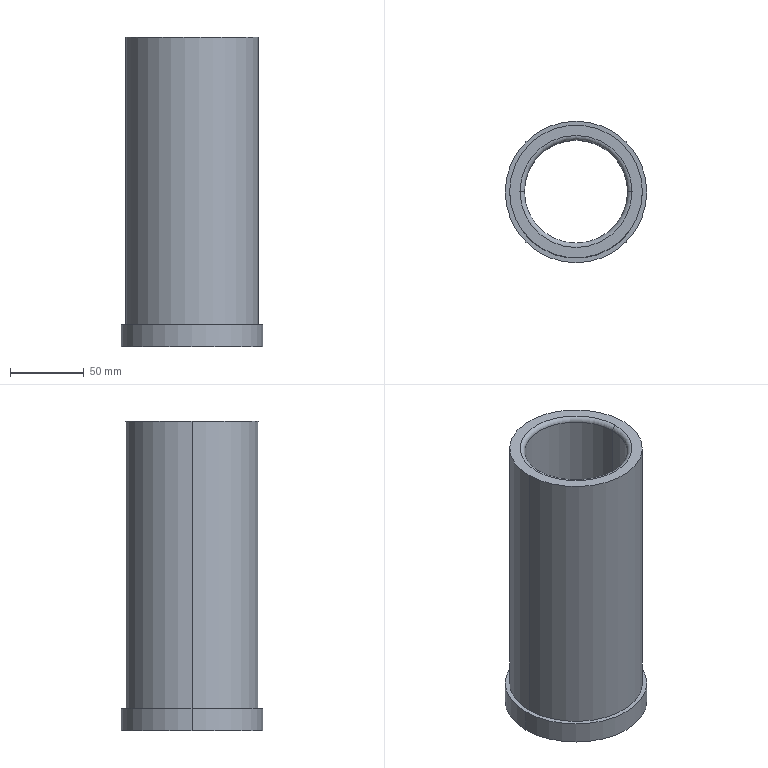Part | SolidWorks | features BaseBody 1 | 1 solid | 13 faces | box 96 x 96 x 210 mm | volume 540069 mm3 | cylinder 6 | torus 4 | plane 3 | commonest cylinder face diameters 70 x2 90 x2 96 x2
STEP:
#1=CARTESIAN_POINT('',(-383.,-275.,-0.5));
#2=VERTEX_POINT('',#1);
#3=CARTESIAN_POINT('',(-307.,-275.,-0.5));
#4=VERTEX_POINT('',#3);
#5=CARTESIAN_POINT('',(-345.,-275.,-0.5));
#6=DIRECTION('',(0.,0.,-1.));
#7=DIRECTION('',(1.,0.,0.));
#8=AXIS2_PLACEMENT_3D('',#5,#6,#7);
#9=CIRCLE('',#8,38.);
#10=EDGE_CURVE('',#2,#4,#9,.T.);
#11=ORIENTED_EDGE('',*,*,#10,.F.);
#12=CARTESIAN_POINT('',(-380.,-275.,-3.5));
#13=VERTEX_POINT('',#12);
#14=CARTESIAN_POINT('',(-383.,-275.,-3.5));
#15=DIRECTION('',(0.,1.,0.));
#16=DIRECTION('',(-1.,0.,0.));
#17=AXIS2_PLACEMENT_3D('',#14,#15,#16);
#18=CIRCLE('',#17,3.);
#19=EDGE_CURVE('',#2,#13,#18,.T.);
#20=ORIENTED_EDGE('',*,*,#19,.T.);
#21=CARTESIAN_POINT('',(-310.,-275.,-3.5));
#22=VERTEX_POINT('',#21);
#23=CARTESIAN_POINT('',(-345.,-275.,-3.5));
#24=DIRECTION('',(0.,0.,1.));
#25=DIRECTION('',(1.,0.,0.));
#26=AXIS2_PLACEMENT_3D('',#23,#24,#25);
#27=CIRCLE('',#26,35.);
#28=EDGE_CURVE('',#22,#13,#27,.T.);
#29=ORIENTED_EDGE('',*,*,#28,.F.);
#30=CARTESIAN_POINT('',(-307.,-275.,-3.5));
#31=DIRECTION('',(0.,-1.,0.));
#32=DIRECTION('',(0.,0.,-1.));
#33=AXIS2_PLACEMENT_3D('',#30,#31,#32);
#34=CIRCLE('',#33,3.);
#35=EDGE_CURVE('',#4,#22,#34,.T.);
#36=ORIENTED_EDGE('',*,*,#35,.F.);
#37=EDGE_LOOP('',(#11,#20,#29,#36));
#38=FACE_OUTER_BOUND('',#37,.T.);
#39=CARTESIAN_POINT('',(-345.,-275.,-3.5));
#40=DIRECTION('',(0.,0.,1.));
#41=DIRECTION('',(1.,0.,0.));
#42=AXIS2_PLACEMENT_3D('',#39,#40,#41);
#43=TOROIDAL_SURFACE('',#42,38.,3.);
#44=ADVANCED_FACE('',(#38),#43,.T.);
#45=CARTESIAN_POINT('',(-380.,-275.,-207.5));
#46=VERTEX_POINT('',#45);
#47=CARTESIAN_POINT('',(-310.,-275.,-207.5));
#48=VERTEX_POINT('',#47);
#49=CARTESIAN_POINT('',(-345.,-275.,-207.5));
#50=DIRECTION('',(0.,0.,-1.));
#51=DIRECTION('',(1.,0.,0.));
#52=AXIS2_PLACEMENT_3D('',#49,#50,#51);
#53=CIRCLE('',#52,35.);
#54=EDGE_CURVE('',#46,#48,#53,.T.);
#55=ORIENTED_EDGE('',*,*,#54,.F.);
#56=CARTESIAN_POINT('',(-383.,-275.,-210.5));
#57=VERTEX_POINT('',#56);
#58=CARTESIAN_POINT('',(-383.,-275.,-207.5));
#59=DIRECTION('',(0.,1.,0.));
#60=DIRECTION('',(-1.,0.,0.));
#61=AXIS2_PLACEMENT_3D('',#58,#59,#60);
#62=CIRCLE('',#61,3.);
#63=EDGE_CURVE('',#46,#57,#62,.T.);
#64=ORIENTED_EDGE('',*,*,#63,.T.);
#65=CARTESIAN_POINT('',(-307.,-275.,-210.5));
#66=VERTEX_POINT('',#65);
#67=CARTESIAN_POINT('',(-345.,-275.,-210.5));
#68=DIRECTION('',(0.,0.,1.));
#69=DIRECTION('',(1.,0.,0.));
#70=AXIS2_PLACEMENT_3D('',#67,#68,#69);
#71=CIRCLE('',#70,38.);
#72=EDGE_CURVE('',#66,#57,#71,.T.);
#73=ORIENTED_EDGE('',*,*,#72,.F.);
#74=CARTESIAN_POINT('',(-307.,-275.,-207.5));
#75=DIRECTION('',(0.,-1.,0.));
#76=DIRECTION('',(0.,0.,-1.));
#77=AXIS2_PLACEMENT_3D('',#74,#75,#76);
#78=CIRCLE('',#77,3.);
#79=EDGE_CURVE('',#48,#66,#78,.T.);
#80=ORIENTED_EDGE('',*,*,#79,.F.);
#81=EDGE_LOOP('',(#55,#64,#73,#80));
#82=FACE_OUTER_BOUND('',#81,.T.);
#83=CARTESIAN_POINT('',(-345.,-275.,-207.5));
#84=DIRECTION('',(0.,0.,1.));
#85=DIRECTION('',(1.,0.,0.));
#86=AXIS2_PLACEMENT_3D('',#83,#84,#85);
#87=TOROIDAL_SURFACE('',#86,38.,3.);
#88=ADVANCED_FACE('',(#82),#87,.T.);
#89=CARTESIAN_POINT('',(-297.,-275.,-210.5));
#90=VERTEX_POINT('',#89);
#91=CARTESIAN_POINT('',(-393.,-275.,-210.5));
#92=VERTEX_POINT('',#91);
#93=CARTESIAN_POINT('',(-345.,-275.,-210.5));
#94=DIRECTION('',(0.,0.,1.));
#95=DIRECTION('',(1.,0.,0.));
#96=AXIS2_PLACEMENT_3D('',#93,#94,#95);
#97=CIRCLE('',#96,48.);
#98=EDGE_CURVE('',#90,#92,#97,.T.);
#99=ORIENTED_EDGE('',*,*,#98,.T.);
#100=CARTESIAN_POINT('',(-393.,-275.,-195.5));
#101=VERTEX_POINT('',#100);
#102=CARTESIAN_POINT('',(-393.,-275.,-210.5));
#103=DIRECTION('',(0.,0.,1.));
#104=VECTOR('',#103,1000.);
#105=LINE('',#102,#104);
#106=EDGE_CURVE('',#92,#101,#105,.T.);
#107=ORIENTED_EDGE('',*,*,#106,.T.);
#108=CARTESIAN_POINT('',(-297.,-275.,-195.5));
#109=VERTEX_POINT('',#108);
#110=CARTESIAN_POINT('',(-345.,-275.,-195.5));
#111=DIRECTION('',(0.,0.,1.));
#112=DIRECTION('',(1.,0.,0.));
#113=AXIS2_PLACEMENT_3D('',#110,#111,#112);
#114=CIRCLE('',#113,48.);
#115=EDGE_CURVE('',#109,#101,#114,.T.);
#116=ORIENTED_EDGE('',*,*,#115,.F.);
#117=CARTESIAN_POINT('',(-297.,-275.,-210.5));
#118=DIRECTION('',(0.,0.,1.));
#119=VECTOR('',#118,1000.);
#120=LINE('',#117,#119);
#121=EDGE_CURVE('',#90,#109,#120,.T.);
#122=ORIENTED_EDGE('',*,*,#121,.F.);
#123=EDGE_LOOP('',(#99,#107,#116,#122));
#124=FACE_OUTER_BOUND('',#123,.T.);
#125=CARTESIAN_POINT('',(-345.,-275.,-210.5));
#126=DIRECTION('',(0.,0.,1.));
#127=DIRECTION('',(1.,0.,0.));
#128=AXIS2_PLACEMENT_3D('',#125,#126,#127);
#129=CYLINDRICAL_SURFACE('',#128,48.);
#130=ADVANCED_FACE('',(#124),#129,.T.);
#131=CARTESIAN_POINT('',(-345.,-275.,-207.5));
#132=DIRECTION('',(0.,0.,-1.));
#133=DIRECTION('',(1.,0.,0.));
#134=AXIS2_PLACEMENT_3D('',#131,#132,#133);
#135=CIRCLE('',#134,35.);
#136=EDGE_CURVE('',#48,#46,#135,.T.);
#137=ORIENTED_EDGE('',*,*,#136,.T.);
#138=CARTESIAN_POINT('',(-380.,-275.,-210.5));
#139=DIRECTION('',(0.,0.,1.));
#140=VECTOR('',#139,1000.);
#141=LINE('',#138,#140);
#142=EDGE_CURVE('',#46,#13,#141,.T.);
#143=ORIENTED_EDGE('',*,*,#142,.T.);
#144=CARTESIAN_POINT('',(-345.,-275.,-3.5));
#145=DIRECTION('',(0.,0.,1.));
#146=DIRECTION('',(1.,0.,0.));
#147=AXIS2_PLACEMENT_3D('',#144,#145,#146);
#148=CIRCLE('',#147,35.);
#149=EDGE_CURVE('',#13,#22,#148,.T.);
#150=ORIENTED_EDGE('',*,*,#149,.T.);
#151=CARTESIAN_POINT('',(-310.,-275.,-210.5));
#152=DIRECTION('',(0.,0.,1.));
#153=VECTOR('',#152,1000.);
#154=LINE('',#151,#153);
#155=EDGE_CURVE('',#48,#22,#154,.T.);
#156=ORIENTED_EDGE('',*,*,#155,.F.);
#157=EDGE_LOOP('',(#137,#143,#150,#156));
#158=FACE_OUTER_BOUND('',#157,.T.);
#159=CARTESIAN_POINT('',(-345.,-275.,-210.5));
#160=DIRECTION('',(0.,0.,1.));
#161=DIRECTION('',(1.,0.,0.));
#162=AXIS2_PLACEMENT_3D('',#159,#160,#161);
#163=CYLINDRICAL_SURFACE('',#162,35.);
#164=ADVANCED_FACE('',(#158),#163,.F.);
#165=CARTESIAN_POINT('',(-390.,-275.,-195.5));
#166=VERTEX_POINT('',#165);
#167=CARTESIAN_POINT('',(-300.,-275.,-195.5));
#168=VERTEX_POINT('',#167);
#169=CARTESIAN_POINT('',(-345.,-275.,-195.5));
#170=DIRECTION('',(0.,0.,-1.));
#171=DIRECTION('',(-1.,0.,0.));
#172=AXIS2_PLACEMENT_3D('',#169,#170,#171);
#173=CIRCLE('',#172,45.);
#174=EDGE_CURVE('',#166,#168,#173,.T.);
#175=ORIENTED_EDGE('',*,*,#174,.F.);
#176=CARTESIAN_POINT('',(-390.,-275.,-0.5));
#177=VERTEX_POINT('',#176);
#178=CARTESIAN_POINT('',(-390.,-275.,-210.5));
#179=DIRECTION('',(0.,0.,1.));
#180=VECTOR('',#179,1000.);
#181=LINE('',#178,#180);
#182=EDGE_CURVE('',#166,#177,#181,.T.);
#183=ORIENTED_EDGE('',*,*,#182,.T.);
#184=CARTESIAN_POINT('',(-300.,-275.,-0.5));
#185=VERTEX_POINT('',#184);
#186=CARTESIAN_POINT('',(-345.,-275.,-0.5));
#187=DIRECTION('',(0.,0.,1.));
#188=DIRECTION('',(1.,0.,0.));
#189=AXIS2_PLACEMENT_3D('',#186,#187,#188);
#190=CIRCLE('',#189,45.);
#191=EDGE_CURVE('',#185,#177,#190,.T.);
#192=ORIENTED_EDGE('',*,*,#191,.F.);
#193=CARTESIAN_POINT('',(-300.,-275.,-210.5));
#194=DIRECTION('',(0.,0.,1.));
#195=VECTOR('',#194,1000.);
#196=LINE('',#193,#195);
#197=EDGE_CURVE('',#168,#185,#196,.T.);
#198=ORIENTED_EDGE('',*,*,#197,.F.);
#199=EDGE_LOOP('',(#175,#183,#192,#198));
#200=FACE_OUTER_BOUND('',#199,.T.);
#201=CARTESIAN_POINT('',(-345.,-275.,-210.5));
#202=DIRECTION('',(0.,0.,1.));
#203=DIRECTION('',(1.,0.,0.));
#204=AXIS2_PLACEMENT_3D('',#201,#202,#203);
#205=CYLINDRICAL_SURFACE('',#204,45.);
#206=ADVANCED_FACE('',(#200),#205,.T.);
#207=ORIENTED_EDGE('',*,*,#182,.F.);
#208=CARTESIAN_POINT('',(-345.,-275.,-195.5));
#209=DIRECTION('',(0.,0.,-1.));
#210=DIRECTION('',(-1.,0.,0.));
#211=AXIS2_PLACEMENT_3D('',#208,#209,#210);
#212=CIRCLE('',#211,45.);
#213=EDGE_CURVE('',#168,#166,#212,.T.);
#214=ORIENTED_EDGE('',*,*,#213,.F.);
#215=ORIENTED_EDGE('',*,*,#197,.T.);
#216=CARTESIAN_POINT('',(-345.,-275.,-0.5));
#217=DIRECTION('',(0.,0.,1.));
#218=DIRECTION('',(1.,0.,0.));
#219=AXIS2_PLACEMENT_3D('',#216,#217,#218);
#220=CIRCLE('',#219,45.);
#221=EDGE_CURVE('',#177,#185,#220,.T.);
#222=ORIENTED_EDGE('',*,*,#221,.F.);
#223=EDGE_LOOP('',(#207,#214,#215,#222));
#224=FACE_OUTER_BOUND('',#223,.T.);
#225=CARTESIAN_POINT('',(-345.,-275.,-210.5));
#226=DIRECTION('',(0.,0.,1.));
#227=DIRECTION('',(1.,0.,0.));
#228=AXIS2_PLACEMENT_3D('',#225,#226,#227);
#229=CYLINDRICAL_SURFACE('',#228,45.);
#230=ADVANCED_FACE('',(#224),#229,.T.);
#231=ORIENTED_EDGE('',*,*,#142,.F.);
#232=ORIENTED_EDGE('',*,*,#54,.T.);
#233=ORIENTED_EDGE('',*,*,#155,.T.);
#234=ORIENTED_EDGE('',*,*,#28,.T.);
#235=EDGE_LOOP('',(#231,#232,#233,#234));
#236=FACE_OUTER_BOUND('',#235,.T.);
#237=CARTESIAN_POINT('',(-345.,-275.,-210.5));
#238=DIRECTION('',(0.,0.,1.));
#239=DIRECTION('',(1.,0.,0.));
#240=AXIS2_PLACEMENT_3D('',#237,#238,#239);
#241=CYLINDRICAL_SURFACE('',#240,35.);
#242=ADVANCED_FACE('',(#236),#241,.F.);
#243=ORIENTED_EDGE('',*,*,#72,.T.);
#244=CARTESIAN_POINT('',(-345.,-275.,-210.5));
#245=DIRECTION('',(0.,0.,1.));
#246=DIRECTION('',(1.,0.,0.));
#247=AXIS2_PLACEMENT_3D('',#244,#245,#246);
#248=CIRCLE('',#247,38.);
#249=EDGE_CURVE('',#57,#66,#248,.T.);
#250=ORIENTED_EDGE('',*,*,#249,.T.);
#251=EDGE_LOOP('',(#243,#250));
#252=FACE_BOUND('',#251,.T.);
#253=ORIENTED_EDGE('',*,*,#98,.F.);
#254=CARTESIAN_POINT('',(-345.,-275.,-210.5));
#255=DIRECTION('',(0.,0.,1.));
#256=DIRECTION('',(1.,0.,0.));
#257=AXIS2_PLACEMENT_3D('',#254,#255,#256);
#258=CIRCLE('',#257,48.);
#259=EDGE_CURVE('',#92,#90,#258,.T.);
#260=ORIENTED_EDGE('',*,*,#259,.F.);
#261=EDGE_LOOP('',(#253,#260));
#262=FACE_OUTER_BOUND('',#261,.T.);
#263=CARTESIAN_POINT('',(-345.,-275.,-210.5));
#264=DIRECTION('',(0.,0.,1.));
#265=DIRECTION('',(1.,0.,0.));
#266=AXIS2_PLACEMENT_3D('',#263,#264,#265);
#267=PLANE('',#266);
#268=ADVANCED_FACE('',(#252,#262),#267,.F.);
#269=CARTESIAN_POINT('',(-345.,-275.,-0.5));
#270=DIRECTION('',(0.,0.,-1.));
#271=DIRECTION('',(1.,0.,0.));
#272=AXIS2_PLACEMENT_3D('',#269,#270,#271);
#273=CIRCLE('',#272,38.);
#274=EDGE_CURVE('',#4,#2,#273,.T.);
#275=ORIENTED_EDGE('',*,*,#274,.T.);
#276=ORIENTED_EDGE('',*,*,#10,.T.);
#277=EDGE_LOOP('',(#275,#276));
#278=FACE_BOUND('',#277,.T.);
#279=ORIENTED_EDGE('',*,*,#191,.T.);
#280=ORIENTED_EDGE('',*,*,#221,.T.);
#281=EDGE_LOOP('',(#279,#280));
#282=FACE_OUTER_BOUND('',#281,.T.);
#283=CARTESIAN_POINT('',(-345.,-275.,-0.5));
#284=DIRECTION('',(0.,0.,1.));
#285=DIRECTION('',(1.,0.,0.));
#286=AXIS2_PLACEMENT_3D('',#283,#284,#285);
#287=PLANE('',#286);
#288=ADVANCED_FACE('',(#278,#282),#287,.T.);
#289=ORIENTED_EDGE('',*,*,#106,.F.);
#290=ORIENTED_EDGE('',*,*,#259,.T.);
#291=ORIENTED_EDGE('',*,*,#121,.T.);
#292=CARTESIAN_POINT('',(-345.,-275.,-195.5));
#293=DIRECTION('',(0.,0.,1.));
#294=DIRECTION('',(1.,0.,0.));
#295=AXIS2_PLACEMENT_3D('',#292,#293,#294);
#296=CIRCLE('',#295,48.);
#297=EDGE_CURVE('',#101,#109,#296,.T.);
#298=ORIENTED_EDGE('',*,*,#297,.F.);
#299=EDGE_LOOP('',(#289,#290,#291,#298));
#300=FACE_OUTER_BOUND('',#299,.T.);
#301=CARTESIAN_POINT('',(-345.,-275.,-210.5));
#302=DIRECTION('',(0.,0.,1.));
#303=DIRECTION('',(1.,0.,0.));
#304=AXIS2_PLACEMENT_3D('',#301,#302,#303);
#305=CYLINDRICAL_SURFACE('',#304,48.);
#306=ADVANCED_FACE('',(#300),#305,.T.);
#307=ORIENTED_EDGE('',*,*,#115,.T.);
#308=ORIENTED_EDGE('',*,*,#297,.T.);
#309=EDGE_LOOP('',(#307,#308));
#310=FACE_OUTER_BOUND('',#309,.T.);
#311=ORIENTED_EDGE('',*,*,#213,.T.);
#312=ORIENTED_EDGE('',*,*,#174,.T.);
#313=EDGE_LOOP('',(#311,#312));
#314=FACE_BOUND('',#313,.T.);
#315=CARTESIAN_POINT('',(-345.,-275.,-195.5));
#316=DIRECTION('',(0.,0.,-1.));
#317=DIRECTION('',(-1.,0.,0.));
#318=AXIS2_PLACEMENT_3D('',#315,#316,#317);
#319=PLANE('',#318);
#320=ADVANCED_FACE('',(#310,#314),#319,.F.);
#321=ORIENTED_EDGE('',*,*,#63,.F.);
#322=ORIENTED_EDGE('',*,*,#136,.F.);
#323=ORIENTED_EDGE('',*,*,#79,.T.);
#324=ORIENTED_EDGE('',*,*,#249,.F.);
#325=EDGE_LOOP('',(#321,#322,#323,#324));
#326=FACE_OUTER_BOUND('',#325,.T.);
#327=CARTESIAN_POINT('',(-345.,-275.,-207.5));
#328=DIRECTION('',(0.,0.,1.));
#329=DIRECTION('',(1.,0.,0.));
#330=AXIS2_PLACEMENT_3D('',#327,#328,#329);
#331=TOROIDAL_SURFACE('',#330,38.,3.);
#332=ADVANCED_FACE('',(#326),#331,.T.);
#333=ORIENTED_EDGE('',*,*,#19,.F.);
#334=ORIENTED_EDGE('',*,*,#274,.F.);
#335=ORIENTED_EDGE('',*,*,#35,.T.);
#336=ORIENTED_EDGE('',*,*,#149,.F.);
#337=EDGE_LOOP('',(#333,#334,#335,#336));
#338=FACE_OUTER_BOUND('',#337,.T.);
#339=CARTESIAN_POINT('',(-345.,-275.,-3.5));
#340=DIRECTION('',(0.,0.,1.));
#341=DIRECTION('',(1.,0.,0.));
#342=AXIS2_PLACEMENT_3D('',#339,#340,#341);
#343=TOROIDAL_SURFACE('',#342,38.,3.);
#344=ADVANCED_FACE('',(#338),#343,.T.);
#345=CLOSED_SHELL('',(#44,#88,#130,#164,#206,#230,#242,#268,#288,#306,#320,#332,#344));
#346=MANIFOLD_SOLID_BREP('',#345);
#347=CARTESIAN_POINT('',(0.,0.,0.));
#348=DIRECTION('',(0.,0.,1.));
#349=DIRECTION('',(1.,0.,0.));
#350=AXIS2_PLACEMENT_3D('',#347,#348,#349);
#351=(LENGTH_UNIT()NAMED_UNIT(*)SI_UNIT(.MILLI.,.METRE.));
#352=UNCERTAINTY_MEASURE_WITH_UNIT(LENGTH_MEASURE(0.00001),#351,'','');
#353=(NAMED_UNIT(*)PLANE_ANGLE_UNIT()SI_UNIT($,.RADIAN.));
#354=(NAMED_UNIT(*)SI_UNIT($,.STERADIAN.)SOLID_ANGLE_UNIT());
#355=(GEOMETRIC_REPRESENTATION_CONTEXT(3)GLOBAL_UNCERTAINTY_ASSIGNED_CONTEXT((#352))GLOBAL_UNIT_ASSIGNED_CONTEXT((#351,#353,#354))REPRESENTATION_CONTEXT('',''));
#356=ADVANCED_BREP_SHAPE_REPRESENTATION('',(#346,#350),#355);